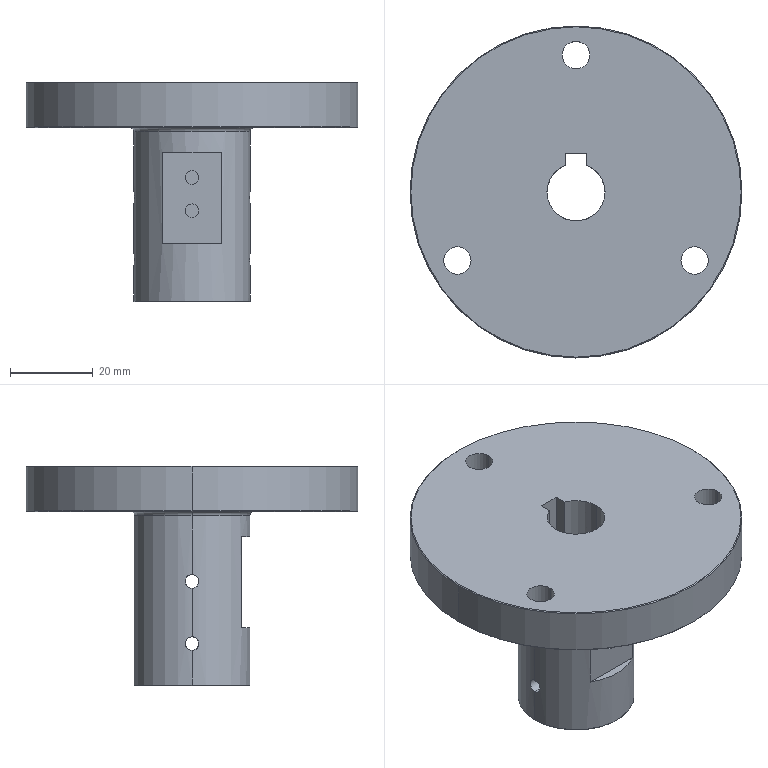Part | SolidWorks | features ICE 4, HoleWzd 3, Chamfer 1, CirPattern 1, Extrusion 1, Fillet 1 | 1 solid | 51 faces | box 80 x 80 x 53 mm | volume 69285 mm3 | cylinder 31 | plane 12 | cone 6 | torus 2 | commonest cylinder face diameters 3.3 x12 6.6 x6 11 x6 14 x3 28 x2 80 x2